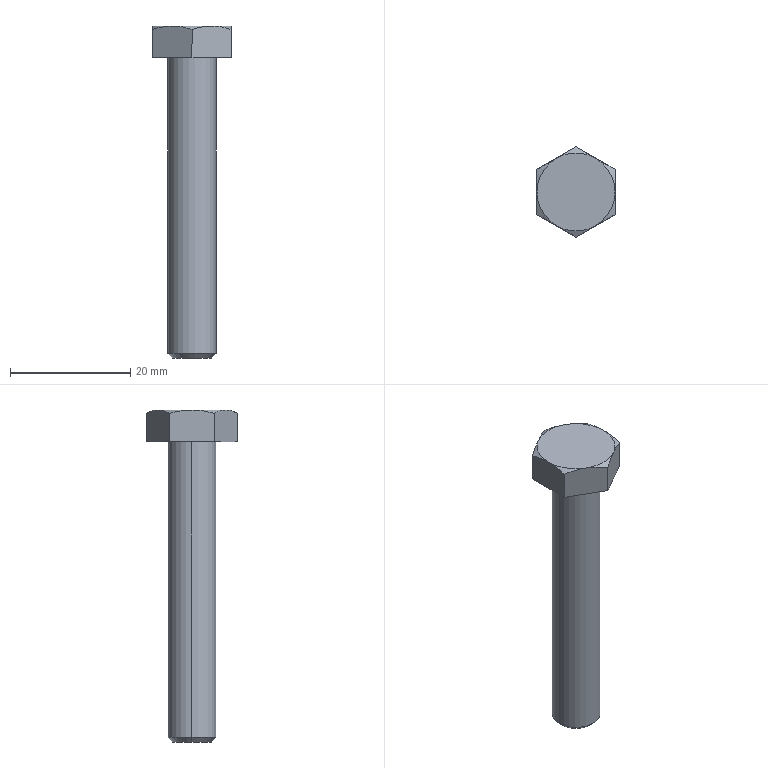Part | SolidWorks | features BaseBody 1 | 1 solid | 19 faces | box 13 x 15.011 x 55.3 mm | volume 3280 mm3 | plane 9 | cone 8 | cylinder 2 | commonest cylinder face diameters 8 x2
STEP:
#1=CARTESIAN_POINT('',(4.,0.,-49.233));
#2=VERTEX_POINT('',#1);
#3=CARTESIAN_POINT('',(-4.,0.,-49.233));
#4=VERTEX_POINT('',#3);
#5=CARTESIAN_POINT('',(0.,0.,-49.233));
#6=DIRECTION('',(0.,0.,1.));
#7=DIRECTION('',(1.,0.,0.));
#8=AXIS2_PLACEMENT_3D('',#5,#6,#7);
#9=CIRCLE('',#8,4.);
#10=EDGE_CURVE('',#2,#4,#9,.T.);
#11=ORIENTED_EDGE('',*,*,#10,.T.);
#12=CARTESIAN_POINT('',(-4.,0.,0.));
#13=VERTEX_POINT('',#12);
#14=CARTESIAN_POINT('',(-4.,0.,-40.));
#15=DIRECTION('',(0.,0.,1.));
#16=VECTOR('',#15,1000.);
#17=LINE('',#14,#16);
#18=EDGE_CURVE('',#4,#13,#17,.T.);
#19=ORIENTED_EDGE('',*,*,#18,.T.);
#20=CARTESIAN_POINT('',(4.,0.,0.));
#21=VERTEX_POINT('',#20);
#22=CARTESIAN_POINT('',(0.,0.,0.));
#23=DIRECTION('',(0.,0.,-1.));
#24=DIRECTION('',(1.,0.,0.));
#25=AXIS2_PLACEMENT_3D('',#22,#23,#24);
#26=CIRCLE('',#25,4.);
#27=EDGE_CURVE('',#13,#21,#26,.T.);
#28=ORIENTED_EDGE('',*,*,#27,.T.);
#29=CARTESIAN_POINT('',(4.,0.,-40.));
#30=DIRECTION('',(0.,0.,1.));
#31=VECTOR('',#30,1000.);
#32=LINE('',#29,#31);
#33=EDGE_CURVE('',#2,#21,#32,.T.);
#34=ORIENTED_EDGE('',*,*,#33,.F.);
#35=EDGE_LOOP('',(#11,#19,#28,#34));
#36=FACE_OUTER_BOUND('',#35,.T.);
#37=CARTESIAN_POINT('',(0.,0.,-40.));
#38=DIRECTION('',(0.,0.,1.));
#39=DIRECTION('',(1.,0.,0.));
#40=AXIS2_PLACEMENT_3D('',#37,#38,#39);
#41=CYLINDRICAL_SURFACE('',#40,4.);
#42=ADVANCED_FACE('',(#36),#41,.T.);
#43=CARTESIAN_POINT('',(3.233,0.,-50.));
#44=VERTEX_POINT('',#43);
#45=CARTESIAN_POINT('',(-3.233,0.,-50.));
#46=VERTEX_POINT('',#45);
#47=CARTESIAN_POINT('',(0.,0.,-50.));
#48=DIRECTION('',(0.,0.,1.));
#49=DIRECTION('',(1.,0.,0.));
#50=AXIS2_PLACEMENT_3D('',#47,#48,#49);
#51=CIRCLE('',#50,3.233);
#52=EDGE_CURVE('',#44,#46,#51,.T.);
#53=ORIENTED_EDGE('',*,*,#52,.T.);
#54=CARTESIAN_POINT('',(-4.,0.,-49.233));
#55=DIRECTION('',(-0.7071,0.,0.7071));
#56=VECTOR('',#55,1000.);
#57=LINE('',#54,#56);
#58=EDGE_CURVE('',#46,#4,#57,.T.);
#59=ORIENTED_EDGE('',*,*,#58,.T.);
#60=ORIENTED_EDGE('',*,*,#10,.F.);
#61=CARTESIAN_POINT('',(4.,0.,-49.233));
#62=DIRECTION('',(0.7071,0.,0.7071));
#63=VECTOR('',#62,1000.);
#64=LINE('',#61,#63);
#65=EDGE_CURVE('',#44,#2,#64,.T.);
#66=ORIENTED_EDGE('',*,*,#65,.F.);
#67=EDGE_LOOP('',(#53,#59,#60,#66));
#68=FACE_OUTER_BOUND('',#67,.T.);
#69=CARTESIAN_POINT('',(0.,0.,-49.233));
#70=DIRECTION('',(0.,0.,1.));
#71=DIRECTION('',(1.,0.,0.));
#72=AXIS2_PLACEMENT_3D('',#69,#70,#71);
#73=CONICAL_SURFACE('',#72,4.,0.7854);
#74=ADVANCED_FACE('',(#68),#73,.T.);
#75=ORIENTED_EDGE('',*,*,#18,.F.);
#76=CARTESIAN_POINT('',(0.,0.,-49.233));
#77=DIRECTION('',(0.,0.,1.));
#78=DIRECTION('',(1.,0.,0.));
#79=AXIS2_PLACEMENT_3D('',#76,#77,#78);
#80=CIRCLE('',#79,4.);
#81=EDGE_CURVE('',#4,#2,#80,.T.);
#82=ORIENTED_EDGE('',*,*,#81,.T.);
#83=ORIENTED_EDGE('',*,*,#33,.T.);
#84=CARTESIAN_POINT('',(0.,0.,0.));
#85=DIRECTION('',(0.,0.,-1.));
#86=DIRECTION('',(1.,0.,0.));
#87=AXIS2_PLACEMENT_3D('',#84,#85,#86);
#88=CIRCLE('',#87,4.);
#89=EDGE_CURVE('',#21,#13,#88,.T.);
#90=ORIENTED_EDGE('',*,*,#89,.T.);
#91=EDGE_LOOP('',(#75,#82,#83,#90));
#92=FACE_OUTER_BOUND('',#91,.T.);
#93=CARTESIAN_POINT('',(0.,0.,-40.));
#94=DIRECTION('',(0.,0.,1.));
#95=DIRECTION('',(1.,0.,0.));
#96=AXIS2_PLACEMENT_3D('',#93,#94,#95);
#97=CYLINDRICAL_SURFACE('',#96,4.);
#98=ADVANCED_FACE('',(#92),#97,.T.);
#99=ORIENTED_EDGE('',*,*,#89,.F.);
#100=ORIENTED_EDGE('',*,*,#27,.F.);
#101=EDGE_LOOP('',(#99,#100));
#102=FACE_BOUND('',#101,.T.);
#103=CARTESIAN_POINT('',(-6.5,3.753,0.));
#104=VERTEX_POINT('',#103);
#105=CARTESIAN_POINT('',(-6.5,-3.753,0.));
#106=VERTEX_POINT('',#105);
#107=CARTESIAN_POINT('',(-6.5,0.,0.));
#108=DIRECTION('',(0.,-1.,0.));
#109=VECTOR('',#108,1000.);
#110=LINE('',#107,#109);
#111=EDGE_CURVE('',#104,#106,#110,.T.);
#112=ORIENTED_EDGE('',*,*,#111,.F.);
#113=CARTESIAN_POINT('',(0.,7.506,0.));
#114=VERTEX_POINT('',#113);
#115=CARTESIAN_POINT('',(0.,7.506,0.));
#116=DIRECTION('',(-0.866,-0.5,0.));
#117=VECTOR('',#116,1000.);
#118=LINE('',#115,#117);
#119=EDGE_CURVE('',#114,#104,#118,.T.);
#120=ORIENTED_EDGE('',*,*,#119,.F.);
#121=CARTESIAN_POINT('',(6.5,3.753,0.));
#122=VERTEX_POINT('',#121);
#123=CARTESIAN_POINT('',(6.5,3.753,0.));
#124=DIRECTION('',(-0.866,0.5,0.));
#125=VECTOR('',#124,1000.);
#126=LINE('',#123,#125);
#127=EDGE_CURVE('',#122,#114,#126,.T.);
#128=ORIENTED_EDGE('',*,*,#127,.F.);
#129=CARTESIAN_POINT('',(6.5,-3.753,0.));
#130=VERTEX_POINT('',#129);
#131=CARTESIAN_POINT('',(6.5,0.,0.));
#132=DIRECTION('',(0.,1.,0.));
#133=VECTOR('',#132,1000.);
#134=LINE('',#131,#133);
#135=EDGE_CURVE('',#130,#122,#134,.T.);
#136=ORIENTED_EDGE('',*,*,#135,.F.);
#137=CARTESIAN_POINT('',(0.,-7.506,0.));
#138=VERTEX_POINT('',#137);
#139=CARTESIAN_POINT('',(0.,-7.506,0.));
#140=DIRECTION('',(0.866,0.5,0.));
#141=VECTOR('',#140,1000.);
#142=LINE('',#139,#141);
#143=EDGE_CURVE('',#138,#130,#142,.T.);
#144=ORIENTED_EDGE('',*,*,#143,.F.);
#145=CARTESIAN_POINT('',(-6.5,-3.753,0.));
#146=DIRECTION('',(0.866,-0.5,0.));
#147=VECTOR('',#146,1000.);
#148=LINE('',#145,#147);
#149=EDGE_CURVE('',#106,#138,#148,.T.);
#150=ORIENTED_EDGE('',*,*,#149,.F.);
#151=EDGE_LOOP('',(#112,#120,#128,#136,#144,#150));
#152=FACE_OUTER_BOUND('',#151,.T.);
#153=CARTESIAN_POINT('',(0.,0.,0.));
#154=DIRECTION('',(0.,0.,1.));
#155=DIRECTION('',(1.,0.,0.));
#156=AXIS2_PLACEMENT_3D('',#153,#154,#155);
#157=PLANE('',#156);
#158=ADVANCED_FACE('',(#102,#152),#157,.F.);
#159=ORIENTED_EDGE('',*,*,#58,.F.);
#160=CARTESIAN_POINT('',(0.,0.,-50.));
#161=DIRECTION('',(0.,0.,1.));
#162=DIRECTION('',(1.,0.,0.));
#163=AXIS2_PLACEMENT_3D('',#160,#161,#162);
#164=CIRCLE('',#163,3.233);
#165=EDGE_CURVE('',#46,#44,#164,.T.);
#166=ORIENTED_EDGE('',*,*,#165,.T.);
#167=ORIENTED_EDGE('',*,*,#65,.T.);
#168=ORIENTED_EDGE('',*,*,#81,.F.);
#169=EDGE_LOOP('',(#159,#166,#167,#168));
#170=FACE_OUTER_BOUND('',#169,.T.);
#171=CARTESIAN_POINT('',(0.,0.,-49.233));
#172=DIRECTION('',(0.,0.,1.));
#173=DIRECTION('',(1.,0.,0.));
#174=AXIS2_PLACEMENT_3D('',#171,#172,#173);
#175=CONICAL_SURFACE('',#174,4.,0.7854);
#176=ADVANCED_FACE('',(#170),#175,.T.);
#177=CARTESIAN_POINT('',(-3.25,-5.629,5.3));
#178=VERTEX_POINT('',#177);
#179=CARTESIAN_POINT('',(0.,-7.506,4.719));
#180=VERTEX_POINT('',#179);
#181=CARTESIAN_POINT('',(-3.25,-5.629,5.3));
#182=CARTESIAN_POINT('',(-2.141,-6.27,5.3));
#183=CARTESIAN_POINT('',(-1.062,-6.892,5.073));
#184=CARTESIAN_POINT('',(0.,-7.506,4.719));
#185=B_SPLINE_CURVE_WITH_KNOTS('',3,(#181,#182,#183,#184),.UNSPECIFIED.,.F.,.F.,(4,4),(0.,0.003797),.UNSPECIFIED.);
#186=EDGE_CURVE('',#178,#180,#185,.T.);
#187=ORIENTED_EDGE('',*,*,#186,.F.);
#188=CARTESIAN_POINT('',(-6.5,-3.753,4.719));
#189=VERTEX_POINT('',#188);
#190=CARTESIAN_POINT('',(-6.5,-3.753,4.719));
#191=CARTESIAN_POINT('',(-5.438,-4.366,5.073));
#192=CARTESIAN_POINT('',(-4.359,-4.989,5.3));
#193=CARTESIAN_POINT('',(-3.25,-5.629,5.3));
#194=B_SPLINE_CURVE_WITH_KNOTS('',3,(#190,#191,#192,#193),.UNSPECIFIED.,.F.,.F.,(4,4),(0.,0.003797),.UNSPECIFIED.);
#195=EDGE_CURVE('',#189,#178,#194,.T.);
#196=ORIENTED_EDGE('',*,*,#195,.F.);
#197=CARTESIAN_POINT('',(-6.5,-3.753,5.3));
#198=DIRECTION('',(0.,0.,1.));
#199=VECTOR('',#198,1000.);
#200=LINE('',#197,#199);
#201=EDGE_CURVE('',#106,#189,#200,.T.);
#202=ORIENTED_EDGE('',*,*,#201,.F.);
#203=ORIENTED_EDGE('',*,*,#149,.T.);
#204=CARTESIAN_POINT('',(0.,-7.506,5.3));
#205=DIRECTION('',(0.,0.,-1.));
#206=VECTOR('',#205,1000.);
#207=LINE('',#204,#206);
#208=EDGE_CURVE('',#180,#138,#207,.T.);
#209=ORIENTED_EDGE('',*,*,#208,.F.);
#210=EDGE_LOOP('',(#187,#196,#202,#203,#209));
#211=FACE_OUTER_BOUND('',#210,.T.);
#212=CARTESIAN_POINT('',(-6.5,-3.753,5.3));
#213=DIRECTION('',(0.5,0.866,0.));
#214=DIRECTION('',(-0.866,0.5,0.));
#215=AXIS2_PLACEMENT_3D('',#212,#213,#214);
#216=PLANE('',#215);
#217=ADVANCED_FACE('',(#211),#216,.F.);
#218=CARTESIAN_POINT('',(-6.5,0.,5.3));
#219=VERTEX_POINT('',#218);
#220=CARTESIAN_POINT('',(-6.5,0.,5.3));
#221=CARTESIAN_POINT('',(-6.5,-1.281,5.3));
#222=CARTESIAN_POINT('',(-6.5,-2.527,5.073));
#223=CARTESIAN_POINT('',(-6.5,-3.753,4.719));
#224=B_SPLINE_CURVE_WITH_KNOTS('',3,(#220,#221,#222,#223),.UNSPECIFIED.,.F.,.F.,(4,4),(0.,0.003797),.UNSPECIFIED.);
#225=EDGE_CURVE('',#219,#189,#224,.T.);
#226=ORIENTED_EDGE('',*,*,#225,.F.);
#227=CARTESIAN_POINT('',(-6.5,3.753,4.719));
#228=VERTEX_POINT('',#227);
#229=CARTESIAN_POINT('',(-6.5,3.753,4.719));
#230=CARTESIAN_POINT('',(-6.5,2.527,5.073));
#231=CARTESIAN_POINT('',(-6.5,1.281,5.3));
#232=CARTESIAN_POINT('',(-6.5,0.,5.3));
#233=B_SPLINE_CURVE_WITH_KNOTS('',3,(#229,#230,#231,#232),.UNSPECIFIED.,.F.,.F.,(4,4),(0.,0.003797),.UNSPECIFIED.);
#234=EDGE_CURVE('',#228,#219,#233,.T.);
#235=ORIENTED_EDGE('',*,*,#234,.F.);
#236=CARTESIAN_POINT('',(-6.5,3.753,5.3));
#237=DIRECTION('',(0.,0.,1.));
#238=VECTOR('',#237,1000.);
#239=LINE('',#236,#238);
#240=EDGE_CURVE('',#104,#228,#239,.T.);
#241=ORIENTED_EDGE('',*,*,#240,.F.);
#242=ORIENTED_EDGE('',*,*,#111,.T.);
#243=ORIENTED_EDGE('',*,*,#201,.T.);
#244=EDGE_LOOP('',(#226,#235,#241,#242,#243));
#245=FACE_OUTER_BOUND('',#244,.T.);
#246=CARTESIAN_POINT('',(-6.5,3.753,5.3));
#247=DIRECTION('',(1.,0.,0.));
#248=DIRECTION('',(0.,1.,0.));
#249=AXIS2_PLACEMENT_3D('',#246,#247,#248);
#250=PLANE('',#249);
#251=ADVANCED_FACE('',(#245),#250,.F.);
#252=CARTESIAN_POINT('',(-3.25,5.629,5.3));
#253=VERTEX_POINT('',#252);
#254=CARTESIAN_POINT('',(-3.25,5.629,5.3));
#255=CARTESIAN_POINT('',(-4.359,4.989,5.3));
#256=CARTESIAN_POINT('',(-5.438,4.366,5.073));
#257=CARTESIAN_POINT('',(-6.5,3.753,4.719));
#258=B_SPLINE_CURVE_WITH_KNOTS('',3,(#254,#255,#256,#257),.UNSPECIFIED.,.F.,.F.,(4,4),(0.,0.003797),.UNSPECIFIED.);
#259=EDGE_CURVE('',#253,#228,#258,.T.);
#260=ORIENTED_EDGE('',*,*,#259,.F.);
#261=CARTESIAN_POINT('',(0.,7.506,4.719));
#262=VERTEX_POINT('',#261);
#263=CARTESIAN_POINT('',(0.,7.506,4.719));
#264=CARTESIAN_POINT('',(-1.062,6.892,5.073));
#265=CARTESIAN_POINT('',(-2.141,6.27,5.3));
#266=CARTESIAN_POINT('',(-3.25,5.629,5.3));
#267=B_SPLINE_CURVE_WITH_KNOTS('',3,(#263,#264,#265,#266),.UNSPECIFIED.,.F.,.F.,(4,4),(0.,0.003797),.UNSPECIFIED.);
#268=EDGE_CURVE('',#262,#253,#267,.T.);
#269=ORIENTED_EDGE('',*,*,#268,.F.);
#270=CARTESIAN_POINT('',(0.,7.506,5.3));
#271=DIRECTION('',(0.,0.,1.));
#272=VECTOR('',#271,1000.);
#273=LINE('',#270,#272);
#274=EDGE_CURVE('',#114,#262,#273,.T.);
#275=ORIENTED_EDGE('',*,*,#274,.F.);
#276=ORIENTED_EDGE('',*,*,#119,.T.);
#277=ORIENTED_EDGE('',*,*,#240,.T.);
#278=EDGE_LOOP('',(#260,#269,#275,#276,#277));
#279=FACE_OUTER_BOUND('',#278,.T.);
#280=CARTESIAN_POINT('',(0.,7.506,5.3));
#281=DIRECTION('',(0.5,-0.866,0.));
#282=DIRECTION('',(0.866,0.5,0.));
#283=AXIS2_PLACEMENT_3D('',#280,#281,#282);
#284=PLANE('',#283);
#285=ADVANCED_FACE('',(#279),#284,.F.);
#286=CARTESIAN_POINT('',(3.25,5.629,5.3));
#287=VERTEX_POINT('',#286);
#288=CARTESIAN_POINT('',(3.25,5.629,5.3));
#289=CARTESIAN_POINT('',(2.141,6.27,5.3));
#290=CARTESIAN_POINT('',(1.062,6.892,5.073));
#291=CARTESIAN_POINT('',(0.,7.506,4.719));
#292=B_SPLINE_CURVE_WITH_KNOTS('',3,(#288,#289,#290,#291),.UNSPECIFIED.,.F.,.F.,(4,4),(0.,0.003797),.UNSPECIFIED.);
#293=EDGE_CURVE('',#287,#262,#292,.T.);
#294=ORIENTED_EDGE('',*,*,#293,.F.);
#295=CARTESIAN_POINT('',(6.5,3.753,4.719));
#296=VERTEX_POINT('',#295);
#297=CARTESIAN_POINT('',(6.5,3.753,4.719));
#298=CARTESIAN_POINT('',(5.438,4.366,5.073));
#299=CARTESIAN_POINT('',(4.359,4.989,5.3));
#300=CARTESIAN_POINT('',(3.25,5.629,5.3));
#301=B_SPLINE_CURVE_WITH_KNOTS('',3,(#297,#298,#299,#300),.UNSPECIFIED.,.F.,.F.,(4,4),(0.,0.003797),.UNSPECIFIED.);
#302=EDGE_CURVE('',#296,#287,#301,.T.);
#303=ORIENTED_EDGE('',*,*,#302,.F.);
#304=CARTESIAN_POINT('',(6.5,3.753,5.3));
#305=DIRECTION('',(0.,0.,1.));
#306=VECTOR('',#305,1000.);
#307=LINE('',#304,#306);
#308=EDGE_CURVE('',#122,#296,#307,.T.);
#309=ORIENTED_EDGE('',*,*,#308,.F.);
#310=ORIENTED_EDGE('',*,*,#127,.T.);
#311=ORIENTED_EDGE('',*,*,#274,.T.);
#312=EDGE_LOOP('',(#294,#303,#309,#310,#311));
#313=FACE_OUTER_BOUND('',#312,.T.);
#314=CARTESIAN_POINT('',(6.5,3.753,5.3));
#315=DIRECTION('',(-0.5,-0.866,0.));
#316=DIRECTION('',(0.866,-0.5,0.));
#317=AXIS2_PLACEMENT_3D('',#314,#315,#316);
#318=PLANE('',#317);
#319=ADVANCED_FACE('',(#313),#318,.F.);
#320=CARTESIAN_POINT('',(6.5,0.,5.3));
#321=VERTEX_POINT('',#320);
#322=CARTESIAN_POINT('',(6.5,0.,5.3));
#323=CARTESIAN_POINT('',(6.5,1.281,5.3));
#324=CARTESIAN_POINT('',(6.5,2.527,5.073));
#325=CARTESIAN_POINT('',(6.5,3.753,4.719));
#326=B_SPLINE_CURVE_WITH_KNOTS('',3,(#322,#323,#324,#325),.UNSPECIFIED.,.F.,.F.,(4,4),(0.,0.003797),.UNSPECIFIED.);
#327=EDGE_CURVE('',#321,#296,#326,.T.);
#328=ORIENTED_EDGE('',*,*,#327,.F.);
#329=CARTESIAN_POINT('',(6.5,-3.753,4.719));
#330=VERTEX_POINT('',#329);
#331=CARTESIAN_POINT('',(6.5,-3.753,4.719));
#332=CARTESIAN_POINT('',(6.5,-2.527,5.073));
#333=CARTESIAN_POINT('',(6.5,-1.281,5.3));
#334=CARTESIAN_POINT('',(6.5,0.,5.3));
#335=B_SPLINE_CURVE_WITH_KNOTS('',3,(#331,#332,#333,#334),.UNSPECIFIED.,.F.,.F.,(4,4),(0.,0.003797),.UNSPECIFIED.);
#336=EDGE_CURVE('',#330,#321,#335,.T.);
#337=ORIENTED_EDGE('',*,*,#336,.F.);
#338=CARTESIAN_POINT('',(6.5,-3.753,5.3));
#339=DIRECTION('',(0.,0.,1.));
#340=VECTOR('',#339,1000.);
#341=LINE('',#338,#340);
#342=EDGE_CURVE('',#130,#330,#341,.T.);
#343=ORIENTED_EDGE('',*,*,#342,.F.);
#344=ORIENTED_EDGE('',*,*,#135,.T.);
#345=ORIENTED_EDGE('',*,*,#308,.T.);
#346=EDGE_LOOP('',(#328,#337,#343,#344,#345));
#347=FACE_OUTER_BOUND('',#346,.T.);
#348=CARTESIAN_POINT('',(6.5,-3.753,5.3));
#349=DIRECTION('',(-1.,0.,0.));
#350=DIRECTION('',(0.,-1.,0.));
#351=AXIS2_PLACEMENT_3D('',#348,#349,#350);
#352=PLANE('',#351);
#353=ADVANCED_FACE('',(#347),#352,.F.);
#354=CARTESIAN_POINT('',(3.25,-5.629,5.3));
#355=VERTEX_POINT('',#354);
#356=CARTESIAN_POINT('',(3.25,-5.629,5.3));
#357=CARTESIAN_POINT('',(4.359,-4.989,5.3));
#358=CARTESIAN_POINT('',(5.438,-4.366,5.073));
#359=CARTESIAN_POINT('',(6.5,-3.753,4.719));
#360=B_SPLINE_CURVE_WITH_KNOTS('',3,(#356,#357,#358,#359),.UNSPECIFIED.,.F.,.F.,(4,4),(0.,0.003797),.UNSPECIFIED.);
#361=EDGE_CURVE('',#355,#330,#360,.T.);
#362=ORIENTED_EDGE('',*,*,#361,.F.);
#363=CARTESIAN_POINT('',(0.,-7.506,4.719));
#364=CARTESIAN_POINT('',(1.062,-6.892,5.073));
#365=CARTESIAN_POINT('',(2.141,-6.27,5.3));
#366=CARTESIAN_POINT('',(3.25,-5.629,5.3));
#367=B_SPLINE_CURVE_WITH_KNOTS('',3,(#363,#364,#365,#366),.UNSPECIFIED.,.F.,.F.,(4,4),(0.,0.003797),.UNSPECIFIED.);
#368=EDGE_CURVE('',#180,#355,#367,.T.);
#369=ORIENTED_EDGE('',*,*,#368,.F.);
#370=ORIENTED_EDGE('',*,*,#208,.T.);
#371=ORIENTED_EDGE('',*,*,#143,.T.);
#372=ORIENTED_EDGE('',*,*,#342,.T.);
#373=EDGE_LOOP('',(#362,#369,#370,#371,#372));
#374=FACE_OUTER_BOUND('',#373,.T.);
#375=CARTESIAN_POINT('',(0.,-7.506,5.3));
#376=DIRECTION('',(-0.5,0.866,0.));
#377=DIRECTION('',(-0.866,-0.5,0.));
#378=AXIS2_PLACEMENT_3D('',#375,#376,#377);
#379=PLANE('',#378);
#380=ADVANCED_FACE('',(#374),#379,.F.);
#381=ORIENTED_EDGE('',*,*,#52,.F.);
#382=ORIENTED_EDGE('',*,*,#165,.F.);
#383=EDGE_LOOP('',(#381,#382));
#384=FACE_OUTER_BOUND('',#383,.T.);
#385=CARTESIAN_POINT('',(0.,3.233,-50.));
#386=DIRECTION('',(0.,0.,1.));
#387=DIRECTION('',(1.,0.,0.));
#388=AXIS2_PLACEMENT_3D('',#385,#386,#387);
#389=PLANE('',#388);
#390=ADVANCED_FACE('',(#384),#389,.F.);
#391=ORIENTED_EDGE('',*,*,#186,.T.);
#392=ORIENTED_EDGE('',*,*,#368,.T.);
#393=CARTESIAN_POINT('',(0.,0.,5.3));
#394=DIRECTION('',(0.,0.,-1.));
#395=DIRECTION('',(-1.,0.,0.));
#396=AXIS2_PLACEMENT_3D('',#393,#394,#395);
#397=CIRCLE('',#396,6.5);
#398=EDGE_CURVE('',#355,#178,#397,.T.);
#399=ORIENTED_EDGE('',*,*,#398,.T.);
#400=EDGE_LOOP('',(#391,#392,#399));
#401=FACE_OUTER_BOUND('',#400,.T.);
#402=CARTESIAN_POINT('',(0.,0.,4.716));
#403=DIRECTION('',(0.,0.,-1.));
#404=DIRECTION('',(-1.,0.,0.));
#405=AXIS2_PLACEMENT_3D('',#402,#403,#404);
#406=CONICAL_SURFACE('',#405,7.512,1.047);
#407=ADVANCED_FACE('',(#401),#406,.T.);
#408=ORIENTED_EDGE('',*,*,#225,.T.);
#409=ORIENTED_EDGE('',*,*,#195,.T.);
#410=CARTESIAN_POINT('',(0.,0.,5.3));
#411=DIRECTION('',(0.,0.,-1.));
#412=DIRECTION('',(-1.,0.,0.));
#413=AXIS2_PLACEMENT_3D('',#410,#411,#412);
#414=CIRCLE('',#413,6.5);
#415=EDGE_CURVE('',#178,#219,#414,.T.);
#416=ORIENTED_EDGE('',*,*,#415,.T.);
#417=EDGE_LOOP('',(#408,#409,#416));
#418=FACE_OUTER_BOUND('',#417,.T.);
#419=CARTESIAN_POINT('',(0.,0.,4.716));
#420=DIRECTION('',(0.,0.,-1.));
#421=DIRECTION('',(-1.,0.,0.));
#422=AXIS2_PLACEMENT_3D('',#419,#420,#421);
#423=CONICAL_SURFACE('',#422,7.512,1.047);
#424=ADVANCED_FACE('',(#418),#423,.T.);
#425=CARTESIAN_POINT('',(0.,0.,5.3));
#426=DIRECTION('',(0.,0.,-1.));
#427=DIRECTION('',(-1.,0.,0.));
#428=AXIS2_PLACEMENT_3D('',#425,#426,#427);
#429=CIRCLE('',#428,6.5);
#430=EDGE_CURVE('',#219,#253,#429,.T.);
#431=ORIENTED_EDGE('',*,*,#430,.T.);
#432=ORIENTED_EDGE('',*,*,#259,.T.);
#433=ORIENTED_EDGE('',*,*,#234,.T.);
#434=EDGE_LOOP('',(#431,#432,#433));
#435=FACE_OUTER_BOUND('',#434,.T.);
#436=CARTESIAN_POINT('',(0.,0.,4.716));
#437=DIRECTION('',(0.,0.,-1.));
#438=DIRECTION('',(-1.,0.,0.));
#439=AXIS2_PLACEMENT_3D('',#436,#437,#438);
#440=CONICAL_SURFACE('',#439,7.512,1.047);
#441=ADVANCED_FACE('',(#435),#440,.T.);
#442=ORIENTED_EDGE('',*,*,#268,.T.);
#443=CARTESIAN_POINT('',(0.,0.,5.3));
#444=DIRECTION('',(0.,0.,-1.));
#445=DIRECTION('',(-1.,0.,0.));
#446=AXIS2_PLACEMENT_3D('',#443,#444,#445);
#447=CIRCLE('',#446,6.5);
#448=EDGE_CURVE('',#253,#287,#447,.T.);
#449=ORIENTED_EDGE('',*,*,#448,.T.);
#450=ORIENTED_EDGE('',*,*,#293,.T.);
#451=EDGE_LOOP('',(#442,#449,#450));
#452=FACE_OUTER_BOUND('',#451,.T.);
#453=CARTESIAN_POINT('',(0.,0.,4.716));
#454=DIRECTION('',(0.,0.,-1.));
#455=DIRECTION('',(-1.,0.,0.));
#456=AXIS2_PLACEMENT_3D('',#453,#454,#455);
#457=CONICAL_SURFACE('',#456,7.512,1.047);
#458=ADVANCED_FACE('',(#452),#457,.T.);
#459=CARTESIAN_POINT('',(0.,0.,5.3));
#460=DIRECTION('',(0.,0.,-1.));
#461=DIRECTION('',(-1.,0.,0.));
#462=AXIS2_PLACEMENT_3D('',#459,#460,#461);
#463=CIRCLE('',#462,6.5);
#464=EDGE_CURVE('',#287,#321,#463,.T.);
#465=ORIENTED_EDGE('',*,*,#464,.T.);
#466=ORIENTED_EDGE('',*,*,#327,.T.);
#467=ORIENTED_EDGE('',*,*,#302,.T.);
#468=EDGE_LOOP('',(#465,#466,#467));
#469=FACE_OUTER_BOUND('',#468,.T.);
#470=CARTESIAN_POINT('',(0.,0.,4.716));
#471=DIRECTION('',(0.,0.,-1.));
#472=DIRECTION('',(-1.,0.,0.));
#473=AXIS2_PLACEMENT_3D('',#470,#471,#472);
#474=CONICAL_SURFACE('',#473,7.512,1.047);
#475=ADVANCED_FACE('',(#469),#474,.T.);
#476=ORIENTED_EDGE('',*,*,#361,.T.);
#477=ORIENTED_EDGE('',*,*,#336,.T.);
#478=CARTESIAN_POINT('',(0.,0.,5.3));
#479=DIRECTION('',(0.,0.,-1.));
#480=DIRECTION('',(-1.,0.,0.));
#481=AXIS2_PLACEMENT_3D('',#478,#479,#480);
#482=CIRCLE('',#481,6.5);
#483=EDGE_CURVE('',#321,#355,#482,.T.);
#484=ORIENTED_EDGE('',*,*,#483,.T.);
#485=EDGE_LOOP('',(#476,#477,#484));
#486=FACE_OUTER_BOUND('',#485,.T.);
#487=CARTESIAN_POINT('',(0.,0.,4.716));
#488=DIRECTION('',(0.,0.,-1.));
#489=DIRECTION('',(-1.,0.,0.));
#490=AXIS2_PLACEMENT_3D('',#487,#488,#489);
#491=CONICAL_SURFACE('',#490,7.512,1.047);
#492=ADVANCED_FACE('',(#486),#491,.T.);
#493=ORIENTED_EDGE('',*,*,#430,.F.);
#494=ORIENTED_EDGE('',*,*,#415,.F.);
#495=ORIENTED_EDGE('',*,*,#398,.F.);
#496=ORIENTED_EDGE('',*,*,#483,.F.);
#497=ORIENTED_EDGE('',*,*,#464,.F.);
#498=ORIENTED_EDGE('',*,*,#448,.F.);
#499=EDGE_LOOP('',(#493,#494,#495,#496,#497,#498));
#500=FACE_OUTER_BOUND('',#499,.T.);
#501=CARTESIAN_POINT('',(0.,0.,5.3));
#502=DIRECTION('',(0.,0.,1.));
#503=DIRECTION('',(1.,0.,0.));
#504=AXIS2_PLACEMENT_3D('',#501,#502,#503);
#505=PLANE('',#504);
#506=ADVANCED_FACE('',(#500),#505,.T.);
#507=CLOSED_SHELL('',(#42,#74,#98,#158,#176,#217,#251,#285,#319,#353,#380,#390,#407,#424,#441,#458,#475,#492,#506));
#508=MANIFOLD_SOLID_BREP('',#507);
#509=CARTESIAN_POINT('',(0.,0.,0.));
#510=DIRECTION('',(0.,0.,1.));
#511=DIRECTION('',(1.,0.,0.));
#512=AXIS2_PLACEMENT_3D('',#509,#510,#511);
#513=(LENGTH_UNIT()NAMED_UNIT(*)SI_UNIT(.MILLI.,.METRE.));
#514=UNCERTAINTY_MEASURE_WITH_UNIT(LENGTH_MEASURE(0.00001),#513,'','');
#515=(NAMED_UNIT(*)PLANE_ANGLE_UNIT()SI_UNIT($,.RADIAN.));
#516=(NAMED_UNIT(*)SI_UNIT($,.STERADIAN.)SOLID_ANGLE_UNIT());
#517=(GEOMETRIC_REPRESENTATION_CONTEXT(3)GLOBAL_UNCERTAINTY_ASSIGNED_CONTEXT((#514))GLOBAL_UNIT_ASSIGNED_CONTEXT((#513,#515,#516))REPRESENTATION_CONTEXT('',''));
#518=ADVANCED_BREP_SHAPE_REPRESENTATION('',(#508,#512),#517);